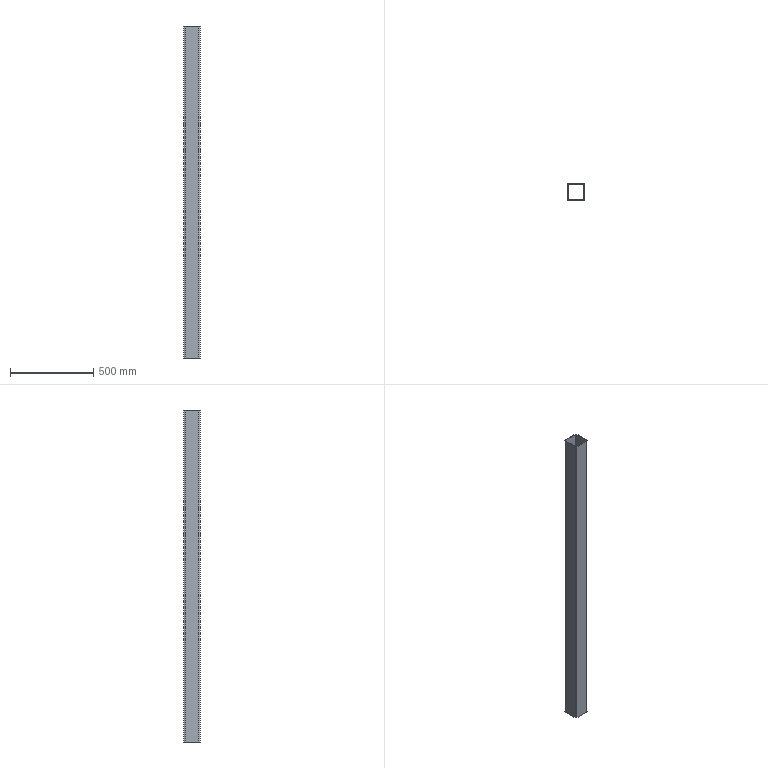Part | SolidWorks | features Extrusion 1, Shell 1 | 1 solid | 18 faces | box 100 x 100 x 2000 mm | volume 2986846 mm3 | plane 10 | cylinder 8 | commonest cylinder face diameters 8.4 x4 16.4 x4
STEP:
#1=CARTESIAN_POINT('',(-50.,-41.8,2000.));
#2=VERTEX_POINT('',#1);
#3=CARTESIAN_POINT('',(-41.8,-50.,2000.));
#4=VERTEX_POINT('',#3);
#5=CARTESIAN_POINT('',(-41.8,-41.8,2000.));
#6=DIRECTION('',(0.,0.,1.));
#7=DIRECTION('',(-1.,0.,0.));
#8=AXIS2_PLACEMENT_3D('',#5,#6,#7);
#9=CIRCLE('',#8,8.2);
#10=EDGE_CURVE('',#2,#4,#9,.T.);
#11=ORIENTED_EDGE('',*,*,#10,.T.);
#12=CARTESIAN_POINT('',(41.8,-50.,2000.));
#13=VERTEX_POINT('',#12);
#14=CARTESIAN_POINT('',(41.8,-50.,2000.));
#15=DIRECTION('',(1.,0.,0.));
#16=VECTOR('',#15,1000.);
#17=LINE('',#14,#16);
#18=EDGE_CURVE('',#4,#13,#17,.T.);
#19=ORIENTED_EDGE('',*,*,#18,.T.);
#20=CARTESIAN_POINT('',(50.,-41.8,2000.));
#21=VERTEX_POINT('',#20);
#22=CARTESIAN_POINT('',(41.8,-41.8,2000.));
#23=DIRECTION('',(0.,0.,1.));
#24=DIRECTION('',(-1.,0.,0.));
#25=AXIS2_PLACEMENT_3D('',#22,#23,#24);
#26=CIRCLE('',#25,8.2);
#27=EDGE_CURVE('',#13,#21,#26,.T.);
#28=ORIENTED_EDGE('',*,*,#27,.T.);
#29=CARTESIAN_POINT('',(50.,41.8,2000.));
#30=VERTEX_POINT('',#29);
#31=CARTESIAN_POINT('',(50.,41.8,2000.));
#32=DIRECTION('',(0.,1.,0.));
#33=VECTOR('',#32,1000.);
#34=LINE('',#31,#33);
#35=EDGE_CURVE('',#21,#30,#34,.T.);
#36=ORIENTED_EDGE('',*,*,#35,.T.);
#37=CARTESIAN_POINT('',(41.8,50.,2000.));
#38=VERTEX_POINT('',#37);
#39=CARTESIAN_POINT('',(41.8,41.8,2000.));
#40=DIRECTION('',(0.,0.,1.));
#41=DIRECTION('',(-1.,0.,0.));
#42=AXIS2_PLACEMENT_3D('',#39,#40,#41);
#43=CIRCLE('',#42,8.2);
#44=EDGE_CURVE('',#30,#38,#43,.T.);
#45=ORIENTED_EDGE('',*,*,#44,.T.);
#46=CARTESIAN_POINT('',(-41.8,50.,2000.));
#47=VERTEX_POINT('',#46);
#48=CARTESIAN_POINT('',(41.8,50.,2000.));
#49=DIRECTION('',(-1.,0.,0.));
#50=VECTOR('',#49,1000.);
#51=LINE('',#48,#50);
#52=EDGE_CURVE('',#38,#47,#51,.T.);
#53=ORIENTED_EDGE('',*,*,#52,.T.);
#54=CARTESIAN_POINT('',(-50.,41.8,2000.));
#55=VERTEX_POINT('',#54);
#56=CARTESIAN_POINT('',(-41.8,41.8,2000.));
#57=DIRECTION('',(0.,0.,1.));
#58=DIRECTION('',(-1.,0.,0.));
#59=AXIS2_PLACEMENT_3D('',#56,#57,#58);
#60=CIRCLE('',#59,8.2);
#61=EDGE_CURVE('',#47,#55,#60,.T.);
#62=ORIENTED_EDGE('',*,*,#61,.T.);
#63=CARTESIAN_POINT('',(-50.,41.8,2000.));
#64=DIRECTION('',(0.,-1.,0.));
#65=VECTOR('',#64,1000.);
#66=LINE('',#63,#65);
#67=EDGE_CURVE('',#55,#2,#66,.T.);
#68=ORIENTED_EDGE('',*,*,#67,.T.);
#69=EDGE_LOOP('',(#11,#19,#28,#36,#45,#53,#62,#68));
#70=FACE_OUTER_BOUND('',#69,.T.);
#71=CARTESIAN_POINT('',(-46.,-41.8,2000.));
#72=VERTEX_POINT('',#71);
#73=CARTESIAN_POINT('',(-41.8,-46.,2000.));
#74=VERTEX_POINT('',#73);
#75=CARTESIAN_POINT('',(-41.8,-41.8,2000.));
#76=DIRECTION('',(0.,0.,1.));
#77=DIRECTION('',(-1.,0.,0.));
#78=AXIS2_PLACEMENT_3D('',#75,#76,#77);
#79=CIRCLE('',#78,4.2);
#80=EDGE_CURVE('',#72,#74,#79,.T.);
#81=ORIENTED_EDGE('',*,*,#80,.F.);
#82=CARTESIAN_POINT('',(-46.,41.8,2000.));
#83=VERTEX_POINT('',#82);
#84=CARTESIAN_POINT('',(-46.,-41.8,2000.));
#85=DIRECTION('',(0.,-1.,0.));
#86=VECTOR('',#85,1000.);
#87=LINE('',#84,#86);
#88=EDGE_CURVE('',#83,#72,#87,.T.);
#89=ORIENTED_EDGE('',*,*,#88,.F.);
#90=CARTESIAN_POINT('',(-41.8,46.,2000.));
#91=VERTEX_POINT('',#90);
#92=CARTESIAN_POINT('',(-41.8,41.8,2000.));
#93=DIRECTION('',(0.,0.,1.));
#94=DIRECTION('',(-1.,0.,0.));
#95=AXIS2_PLACEMENT_3D('',#92,#93,#94);
#96=CIRCLE('',#95,4.2);
#97=EDGE_CURVE('',#91,#83,#96,.T.);
#98=ORIENTED_EDGE('',*,*,#97,.F.);
#99=CARTESIAN_POINT('',(41.8,46.,2000.));
#100=VERTEX_POINT('',#99);
#101=CARTESIAN_POINT('',(-41.8,46.,2000.));
#102=DIRECTION('',(-1.,0.,0.));
#103=VECTOR('',#102,1000.);
#104=LINE('',#101,#103);
#105=EDGE_CURVE('',#100,#91,#104,.T.);
#106=ORIENTED_EDGE('',*,*,#105,.F.);
#107=CARTESIAN_POINT('',(46.,41.8,2000.));
#108=VERTEX_POINT('',#107);
#109=CARTESIAN_POINT('',(41.8,41.8,2000.));
#110=DIRECTION('',(0.,0.,1.));
#111=DIRECTION('',(-1.,0.,0.));
#112=AXIS2_PLACEMENT_3D('',#109,#110,#111);
#113=CIRCLE('',#112,4.2);
#114=EDGE_CURVE('',#108,#100,#113,.T.);
#115=ORIENTED_EDGE('',*,*,#114,.F.);
#116=CARTESIAN_POINT('',(46.,-41.8,2000.));
#117=VERTEX_POINT('',#116);
#118=CARTESIAN_POINT('',(46.,-41.8,2000.));
#119=DIRECTION('',(0.,1.,0.));
#120=VECTOR('',#119,1000.);
#121=LINE('',#118,#120);
#122=EDGE_CURVE('',#117,#108,#121,.T.);
#123=ORIENTED_EDGE('',*,*,#122,.F.);
#124=CARTESIAN_POINT('',(41.8,-46.,2000.));
#125=VERTEX_POINT('',#124);
#126=CARTESIAN_POINT('',(41.8,-41.8,2000.));
#127=DIRECTION('',(0.,0.,1.));
#128=DIRECTION('',(-1.,0.,0.));
#129=AXIS2_PLACEMENT_3D('',#126,#127,#128);
#130=CIRCLE('',#129,4.2);
#131=EDGE_CURVE('',#125,#117,#130,.T.);
#132=ORIENTED_EDGE('',*,*,#131,.F.);
#133=CARTESIAN_POINT('',(-41.8,-46.,2000.));
#134=DIRECTION('',(1.,0.,0.));
#135=VECTOR('',#134,1000.);
#136=LINE('',#133,#135);
#137=EDGE_CURVE('',#74,#125,#136,.T.);
#138=ORIENTED_EDGE('',*,*,#137,.F.);
#139=EDGE_LOOP('',(#81,#89,#98,#106,#115,#123,#132,#138));
#140=FACE_BOUND('',#139,.T.);
#141=CARTESIAN_POINT('',(-41.8,-41.8,2000.));
#142=DIRECTION('',(0.,0.,-1.));
#143=DIRECTION('',(-1.,0.,0.));
#144=AXIS2_PLACEMENT_3D('',#141,#142,#143);
#145=PLANE('',#144);
#146=ADVANCED_FACE('',(#70,#140),#145,.F.);
#147=CARTESIAN_POINT('',(-50.,-41.8,0.));
#148=VERTEX_POINT('',#147);
#149=CARTESIAN_POINT('',(-41.8,-50.,0.));
#150=VERTEX_POINT('',#149);
#151=CARTESIAN_POINT('',(-41.8,-41.8,0.));
#152=DIRECTION('',(0.,0.,1.));
#153=DIRECTION('',(-1.,0.,0.));
#154=AXIS2_PLACEMENT_3D('',#151,#152,#153);
#155=CIRCLE('',#154,8.2);
#156=EDGE_CURVE('',#148,#150,#155,.T.);
#157=ORIENTED_EDGE('',*,*,#156,.F.);
#158=CARTESIAN_POINT('',(-50.,41.8,0.));
#159=VERTEX_POINT('',#158);
#160=CARTESIAN_POINT('',(-50.,41.8,0.));
#161=DIRECTION('',(0.,-1.,0.));
#162=VECTOR('',#161,1000.);
#163=LINE('',#160,#162);
#164=EDGE_CURVE('',#159,#148,#163,.T.);
#165=ORIENTED_EDGE('',*,*,#164,.F.);
#166=CARTESIAN_POINT('',(-41.8,50.,0.));
#167=VERTEX_POINT('',#166);
#168=CARTESIAN_POINT('',(-41.8,41.8,0.));
#169=DIRECTION('',(0.,0.,1.));
#170=DIRECTION('',(-1.,0.,0.));
#171=AXIS2_PLACEMENT_3D('',#168,#169,#170);
#172=CIRCLE('',#171,8.2);
#173=EDGE_CURVE('',#167,#159,#172,.T.);
#174=ORIENTED_EDGE('',*,*,#173,.F.);
#175=CARTESIAN_POINT('',(41.8,50.,0.));
#176=VERTEX_POINT('',#175);
#177=CARTESIAN_POINT('',(41.8,50.,0.));
#178=DIRECTION('',(-1.,0.,0.));
#179=VECTOR('',#178,1000.);
#180=LINE('',#177,#179);
#181=EDGE_CURVE('',#176,#167,#180,.T.);
#182=ORIENTED_EDGE('',*,*,#181,.F.);
#183=CARTESIAN_POINT('',(50.,41.8,0.));
#184=VERTEX_POINT('',#183);
#185=CARTESIAN_POINT('',(41.8,41.8,0.));
#186=DIRECTION('',(0.,0.,1.));
#187=DIRECTION('',(-1.,0.,0.));
#188=AXIS2_PLACEMENT_3D('',#185,#186,#187);
#189=CIRCLE('',#188,8.2);
#190=EDGE_CURVE('',#184,#176,#189,.T.);
#191=ORIENTED_EDGE('',*,*,#190,.F.);
#192=CARTESIAN_POINT('',(50.,-41.8,0.));
#193=VERTEX_POINT('',#192);
#194=CARTESIAN_POINT('',(50.,41.8,0.));
#195=DIRECTION('',(0.,1.,0.));
#196=VECTOR('',#195,1000.);
#197=LINE('',#194,#196);
#198=EDGE_CURVE('',#193,#184,#197,.T.);
#199=ORIENTED_EDGE('',*,*,#198,.F.);
#200=CARTESIAN_POINT('',(41.8,-50.,0.));
#201=VERTEX_POINT('',#200);
#202=CARTESIAN_POINT('',(41.8,-41.8,0.));
#203=DIRECTION('',(0.,0.,1.));
#204=DIRECTION('',(-1.,0.,0.));
#205=AXIS2_PLACEMENT_3D('',#202,#203,#204);
#206=CIRCLE('',#205,8.2);
#207=EDGE_CURVE('',#201,#193,#206,.T.);
#208=ORIENTED_EDGE('',*,*,#207,.F.);
#209=CARTESIAN_POINT('',(41.8,-50.,0.));
#210=DIRECTION('',(1.,0.,0.));
#211=VECTOR('',#210,1000.);
#212=LINE('',#209,#211);
#213=EDGE_CURVE('',#150,#201,#212,.T.);
#214=ORIENTED_EDGE('',*,*,#213,.F.);
#215=EDGE_LOOP('',(#157,#165,#174,#182,#191,#199,#208,#214));
#216=FACE_OUTER_BOUND('',#215,.T.);
#217=CARTESIAN_POINT('',(-46.,41.8,0.));
#218=VERTEX_POINT('',#217);
#219=CARTESIAN_POINT('',(-46.,-41.8,0.));
#220=VERTEX_POINT('',#219);
#221=CARTESIAN_POINT('',(-46.,-41.8,0.));
#222=DIRECTION('',(0.,-1.,0.));
#223=VECTOR('',#222,1000.);
#224=LINE('',#221,#223);
#225=EDGE_CURVE('',#218,#220,#224,.T.);
#226=ORIENTED_EDGE('',*,*,#225,.T.);
#227=CARTESIAN_POINT('',(-41.8,-46.,0.));
#228=VERTEX_POINT('',#227);
#229=CARTESIAN_POINT('',(-41.8,-41.8,0.));
#230=DIRECTION('',(0.,0.,1.));
#231=DIRECTION('',(-1.,0.,0.));
#232=AXIS2_PLACEMENT_3D('',#229,#230,#231);
#233=CIRCLE('',#232,4.2);
#234=EDGE_CURVE('',#220,#228,#233,.T.);
#235=ORIENTED_EDGE('',*,*,#234,.T.);
#236=CARTESIAN_POINT('',(41.8,-46.,0.));
#237=VERTEX_POINT('',#236);
#238=CARTESIAN_POINT('',(-41.8,-46.,0.));
#239=DIRECTION('',(1.,0.,0.));
#240=VECTOR('',#239,1000.);
#241=LINE('',#238,#240);
#242=EDGE_CURVE('',#228,#237,#241,.T.);
#243=ORIENTED_EDGE('',*,*,#242,.T.);
#244=CARTESIAN_POINT('',(46.,-41.8,0.));
#245=VERTEX_POINT('',#244);
#246=CARTESIAN_POINT('',(41.8,-41.8,0.));
#247=DIRECTION('',(0.,0.,1.));
#248=DIRECTION('',(-1.,0.,0.));
#249=AXIS2_PLACEMENT_3D('',#246,#247,#248);
#250=CIRCLE('',#249,4.2);
#251=EDGE_CURVE('',#237,#245,#250,.T.);
#252=ORIENTED_EDGE('',*,*,#251,.T.);
#253=CARTESIAN_POINT('',(46.,41.8,0.));
#254=VERTEX_POINT('',#253);
#255=CARTESIAN_POINT('',(46.,-41.8,0.));
#256=DIRECTION('',(0.,1.,0.));
#257=VECTOR('',#256,1000.);
#258=LINE('',#255,#257);
#259=EDGE_CURVE('',#245,#254,#258,.T.);
#260=ORIENTED_EDGE('',*,*,#259,.T.);
#261=CARTESIAN_POINT('',(41.8,46.,0.));
#262=VERTEX_POINT('',#261);
#263=CARTESIAN_POINT('',(41.8,41.8,0.));
#264=DIRECTION('',(0.,0.,1.));
#265=DIRECTION('',(-1.,0.,0.));
#266=AXIS2_PLACEMENT_3D('',#263,#264,#265);
#267=CIRCLE('',#266,4.2);
#268=EDGE_CURVE('',#254,#262,#267,.T.);
#269=ORIENTED_EDGE('',*,*,#268,.T.);
#270=CARTESIAN_POINT('',(-41.8,46.,0.));
#271=VERTEX_POINT('',#270);
#272=CARTESIAN_POINT('',(-41.8,46.,0.));
#273=DIRECTION('',(-1.,0.,0.));
#274=VECTOR('',#273,1000.);
#275=LINE('',#272,#274);
#276=EDGE_CURVE('',#262,#271,#275,.T.);
#277=ORIENTED_EDGE('',*,*,#276,.T.);
#278=CARTESIAN_POINT('',(-41.8,41.8,0.));
#279=DIRECTION('',(0.,0.,1.));
#280=DIRECTION('',(-1.,0.,0.));
#281=AXIS2_PLACEMENT_3D('',#278,#279,#280);
#282=CIRCLE('',#281,4.2);
#283=EDGE_CURVE('',#271,#218,#282,.T.);
#284=ORIENTED_EDGE('',*,*,#283,.T.);
#285=EDGE_LOOP('',(#226,#235,#243,#252,#260,#269,#277,#284));
#286=FACE_BOUND('',#285,.T.);
#287=CARTESIAN_POINT('',(-41.8,-41.8,0.));
#288=DIRECTION('',(0.,0.,-1.));
#289=DIRECTION('',(-1.,0.,0.));
#290=AXIS2_PLACEMENT_3D('',#287,#288,#289);
#291=PLANE('',#290);
#292=ADVANCED_FACE('',(#216,#286),#291,.T.);
#293=ORIENTED_EDGE('',*,*,#156,.T.);
#294=CARTESIAN_POINT('',(-41.8,-50.,2000.));
#295=DIRECTION('',(0.,0.,-1.));
#296=VECTOR('',#295,1000.);
#297=LINE('',#294,#296);
#298=EDGE_CURVE('',#4,#150,#297,.T.);
#299=ORIENTED_EDGE('',*,*,#298,.F.);
#300=ORIENTED_EDGE('',*,*,#10,.F.);
#301=CARTESIAN_POINT('',(-50.,-41.8,2000.));
#302=DIRECTION('',(0.,0.,-1.));
#303=VECTOR('',#302,1000.);
#304=LINE('',#301,#303);
#305=EDGE_CURVE('',#2,#148,#304,.T.);
#306=ORIENTED_EDGE('',*,*,#305,.T.);
#307=EDGE_LOOP('',(#293,#299,#300,#306));
#308=FACE_OUTER_BOUND('',#307,.T.);
#309=CARTESIAN_POINT('',(-41.8,-41.8,2000.));
#310=DIRECTION('',(0.,0.,-1.));
#311=DIRECTION('',(-1.,0.,0.));
#312=AXIS2_PLACEMENT_3D('',#309,#310,#311);
#313=CYLINDRICAL_SURFACE('',#312,8.2);
#314=ADVANCED_FACE('',(#308),#313,.T.);
#315=ORIENTED_EDGE('',*,*,#213,.T.);
#316=CARTESIAN_POINT('',(41.8,-50.,2000.));
#317=DIRECTION('',(0.,0.,-1.));
#318=VECTOR('',#317,1000.);
#319=LINE('',#316,#318);
#320=EDGE_CURVE('',#13,#201,#319,.T.);
#321=ORIENTED_EDGE('',*,*,#320,.F.);
#322=ORIENTED_EDGE('',*,*,#18,.F.);
#323=ORIENTED_EDGE('',*,*,#298,.T.);
#324=EDGE_LOOP('',(#315,#321,#322,#323));
#325=FACE_OUTER_BOUND('',#324,.T.);
#326=CARTESIAN_POINT('',(41.8,-50.,2000.));
#327=DIRECTION('',(0.,1.,0.));
#328=DIRECTION('',(-1.,0.,0.));
#329=AXIS2_PLACEMENT_3D('',#326,#327,#328);
#330=PLANE('',#329);
#331=ADVANCED_FACE('',(#325),#330,.F.);
#332=ORIENTED_EDGE('',*,*,#207,.T.);
#333=CARTESIAN_POINT('',(50.,-41.8,2000.));
#334=DIRECTION('',(0.,0.,-1.));
#335=VECTOR('',#334,1000.);
#336=LINE('',#333,#335);
#337=EDGE_CURVE('',#21,#193,#336,.T.);
#338=ORIENTED_EDGE('',*,*,#337,.F.);
#339=ORIENTED_EDGE('',*,*,#27,.F.);
#340=ORIENTED_EDGE('',*,*,#320,.T.);
#341=EDGE_LOOP('',(#332,#338,#339,#340));
#342=FACE_OUTER_BOUND('',#341,.T.);
#343=CARTESIAN_POINT('',(41.8,-41.8,2000.));
#344=DIRECTION('',(0.,0.,-1.));
#345=DIRECTION('',(-1.,0.,0.));
#346=AXIS2_PLACEMENT_3D('',#343,#344,#345);
#347=CYLINDRICAL_SURFACE('',#346,8.2);
#348=ADVANCED_FACE('',(#342),#347,.T.);
#349=ORIENTED_EDGE('',*,*,#198,.T.);
#350=CARTESIAN_POINT('',(50.,41.8,2000.));
#351=DIRECTION('',(0.,0.,-1.));
#352=VECTOR('',#351,1000.);
#353=LINE('',#350,#352);
#354=EDGE_CURVE('',#30,#184,#353,.T.);
#355=ORIENTED_EDGE('',*,*,#354,.F.);
#356=ORIENTED_EDGE('',*,*,#35,.F.);
#357=ORIENTED_EDGE('',*,*,#337,.T.);
#358=EDGE_LOOP('',(#349,#355,#356,#357));
#359=FACE_OUTER_BOUND('',#358,.T.);
#360=CARTESIAN_POINT('',(50.,41.8,2000.));
#361=DIRECTION('',(-1.,0.,0.));
#362=DIRECTION('',(0.,-1.,0.));
#363=AXIS2_PLACEMENT_3D('',#360,#361,#362);
#364=PLANE('',#363);
#365=ADVANCED_FACE('',(#359),#364,.F.);
#366=ORIENTED_EDGE('',*,*,#190,.T.);
#367=CARTESIAN_POINT('',(41.8,50.,2000.));
#368=DIRECTION('',(0.,0.,-1.));
#369=VECTOR('',#368,1000.);
#370=LINE('',#367,#369);
#371=EDGE_CURVE('',#38,#176,#370,.T.);
#372=ORIENTED_EDGE('',*,*,#371,.F.);
#373=ORIENTED_EDGE('',*,*,#44,.F.);
#374=ORIENTED_EDGE('',*,*,#354,.T.);
#375=EDGE_LOOP('',(#366,#372,#373,#374));
#376=FACE_OUTER_BOUND('',#375,.T.);
#377=CARTESIAN_POINT('',(41.8,41.8,2000.));
#378=DIRECTION('',(0.,0.,-1.));
#379=DIRECTION('',(-1.,0.,0.));
#380=AXIS2_PLACEMENT_3D('',#377,#378,#379);
#381=CYLINDRICAL_SURFACE('',#380,8.2);
#382=ADVANCED_FACE('',(#376),#381,.T.);
#383=ORIENTED_EDGE('',*,*,#181,.T.);
#384=CARTESIAN_POINT('',(-41.8,50.,2000.));
#385=DIRECTION('',(0.,0.,-1.));
#386=VECTOR('',#385,1000.);
#387=LINE('',#384,#386);
#388=EDGE_CURVE('',#47,#167,#387,.T.);
#389=ORIENTED_EDGE('',*,*,#388,.F.);
#390=ORIENTED_EDGE('',*,*,#52,.F.);
#391=ORIENTED_EDGE('',*,*,#371,.T.);
#392=EDGE_LOOP('',(#383,#389,#390,#391));
#393=FACE_OUTER_BOUND('',#392,.T.);
#394=CARTESIAN_POINT('',(41.8,50.,2000.));
#395=DIRECTION('',(0.,-1.,0.));
#396=DIRECTION('',(1.,0.,0.));
#397=AXIS2_PLACEMENT_3D('',#394,#395,#396);
#398=PLANE('',#397);
#399=ADVANCED_FACE('',(#393),#398,.F.);
#400=ORIENTED_EDGE('',*,*,#173,.T.);
#401=CARTESIAN_POINT('',(-50.,41.8,2000.));
#402=DIRECTION('',(0.,0.,-1.));
#403=VECTOR('',#402,1000.);
#404=LINE('',#401,#403);
#405=EDGE_CURVE('',#55,#159,#404,.T.);
#406=ORIENTED_EDGE('',*,*,#405,.F.);
#407=ORIENTED_EDGE('',*,*,#61,.F.);
#408=ORIENTED_EDGE('',*,*,#388,.T.);
#409=EDGE_LOOP('',(#400,#406,#407,#408));
#410=FACE_OUTER_BOUND('',#409,.T.);
#411=CARTESIAN_POINT('',(-41.8,41.8,2000.));
#412=DIRECTION('',(0.,0.,-1.));
#413=DIRECTION('',(-1.,0.,0.));
#414=AXIS2_PLACEMENT_3D('',#411,#412,#413);
#415=CYLINDRICAL_SURFACE('',#414,8.2);
#416=ADVANCED_FACE('',(#410),#415,.T.);
#417=ORIENTED_EDGE('',*,*,#164,.T.);
#418=ORIENTED_EDGE('',*,*,#305,.F.);
#419=ORIENTED_EDGE('',*,*,#67,.F.);
#420=ORIENTED_EDGE('',*,*,#405,.T.);
#421=EDGE_LOOP('',(#417,#418,#419,#420));
#422=FACE_OUTER_BOUND('',#421,.T.);
#423=CARTESIAN_POINT('',(-50.,41.8,2000.));
#424=DIRECTION('',(1.,0.,0.));
#425=DIRECTION('',(0.,1.,0.));
#426=AXIS2_PLACEMENT_3D('',#423,#424,#425);
#427=PLANE('',#426);
#428=ADVANCED_FACE('',(#422),#427,.F.);
#429=ORIENTED_EDGE('',*,*,#234,.F.);
#430=CARTESIAN_POINT('',(-46.,-41.8,2000.));
#431=DIRECTION('',(0.,0.,-1.));
#432=VECTOR('',#431,1000.);
#433=LINE('',#430,#432);
#434=EDGE_CURVE('',#72,#220,#433,.T.);
#435=ORIENTED_EDGE('',*,*,#434,.F.);
#436=ORIENTED_EDGE('',*,*,#80,.T.);
#437=CARTESIAN_POINT('',(-41.8,-46.,2000.));
#438=DIRECTION('',(0.,0.,-1.));
#439=VECTOR('',#438,1000.);
#440=LINE('',#437,#439);
#441=EDGE_CURVE('',#74,#228,#440,.T.);
#442=ORIENTED_EDGE('',*,*,#441,.T.);
#443=EDGE_LOOP('',(#429,#435,#436,#442));
#444=FACE_OUTER_BOUND('',#443,.T.);
#445=CARTESIAN_POINT('',(-41.8,-41.8,2000.));
#446=DIRECTION('',(0.,0.,-1.));
#447=DIRECTION('',(-1.,0.,0.));
#448=AXIS2_PLACEMENT_3D('',#445,#446,#447);
#449=CYLINDRICAL_SURFACE('',#448,4.2);
#450=ADVANCED_FACE('',(#444),#449,.F.);
#451=ORIENTED_EDGE('',*,*,#242,.F.);
#452=ORIENTED_EDGE('',*,*,#441,.F.);
#453=ORIENTED_EDGE('',*,*,#137,.T.);
#454=CARTESIAN_POINT('',(41.8,-46.,2000.));
#455=DIRECTION('',(0.,0.,-1.));
#456=VECTOR('',#455,1000.);
#457=LINE('',#454,#456);
#458=EDGE_CURVE('',#125,#237,#457,.T.);
#459=ORIENTED_EDGE('',*,*,#458,.T.);
#460=EDGE_LOOP('',(#451,#452,#453,#459));
#461=FACE_OUTER_BOUND('',#460,.T.);
#462=CARTESIAN_POINT('',(41.8,-46.,2000.));
#463=DIRECTION('',(0.,1.,0.));
#464=DIRECTION('',(-1.,0.,0.));
#465=AXIS2_PLACEMENT_3D('',#462,#463,#464);
#466=PLANE('',#465);
#467=ADVANCED_FACE('',(#461),#466,.T.);
#468=ORIENTED_EDGE('',*,*,#251,.F.);
#469=ORIENTED_EDGE('',*,*,#458,.F.);
#470=ORIENTED_EDGE('',*,*,#131,.T.);
#471=CARTESIAN_POINT('',(46.,-41.8,2000.));
#472=DIRECTION('',(0.,0.,-1.));
#473=VECTOR('',#472,1000.);
#474=LINE('',#471,#473);
#475=EDGE_CURVE('',#117,#245,#474,.T.);
#476=ORIENTED_EDGE('',*,*,#475,.T.);
#477=EDGE_LOOP('',(#468,#469,#470,#476));
#478=FACE_OUTER_BOUND('',#477,.T.);
#479=CARTESIAN_POINT('',(41.8,-41.8,2000.));
#480=DIRECTION('',(0.,0.,-1.));
#481=DIRECTION('',(-1.,0.,0.));
#482=AXIS2_PLACEMENT_3D('',#479,#480,#481);
#483=CYLINDRICAL_SURFACE('',#482,4.2);
#484=ADVANCED_FACE('',(#478),#483,.F.);
#485=ORIENTED_EDGE('',*,*,#259,.F.);
#486=ORIENTED_EDGE('',*,*,#475,.F.);
#487=ORIENTED_EDGE('',*,*,#122,.T.);
#488=CARTESIAN_POINT('',(46.,41.8,2000.));
#489=DIRECTION('',(0.,0.,-1.));
#490=VECTOR('',#489,1000.);
#491=LINE('',#488,#490);
#492=EDGE_CURVE('',#108,#254,#491,.T.);
#493=ORIENTED_EDGE('',*,*,#492,.T.);
#494=EDGE_LOOP('',(#485,#486,#487,#493));
#495=FACE_OUTER_BOUND('',#494,.T.);
#496=CARTESIAN_POINT('',(46.,41.8,2000.));
#497=DIRECTION('',(-1.,0.,0.));
#498=DIRECTION('',(0.,-1.,0.));
#499=AXIS2_PLACEMENT_3D('',#496,#497,#498);
#500=PLANE('',#499);
#501=ADVANCED_FACE('',(#495),#500,.T.);
#502=ORIENTED_EDGE('',*,*,#268,.F.);
#503=ORIENTED_EDGE('',*,*,#492,.F.);
#504=ORIENTED_EDGE('',*,*,#114,.T.);
#505=CARTESIAN_POINT('',(41.8,46.,2000.));
#506=DIRECTION('',(0.,0.,-1.));
#507=VECTOR('',#506,1000.);
#508=LINE('',#505,#507);
#509=EDGE_CURVE('',#100,#262,#508,.T.);
#510=ORIENTED_EDGE('',*,*,#509,.T.);
#511=EDGE_LOOP('',(#502,#503,#504,#510));
#512=FACE_OUTER_BOUND('',#511,.T.);
#513=CARTESIAN_POINT('',(41.8,41.8,2000.));
#514=DIRECTION('',(0.,0.,-1.));
#515=DIRECTION('',(-1.,0.,0.));
#516=AXIS2_PLACEMENT_3D('',#513,#514,#515);
#517=CYLINDRICAL_SURFACE('',#516,4.2);
#518=ADVANCED_FACE('',(#512),#517,.F.);
#519=ORIENTED_EDGE('',*,*,#276,.F.);
#520=ORIENTED_EDGE('',*,*,#509,.F.);
#521=ORIENTED_EDGE('',*,*,#105,.T.);
#522=CARTESIAN_POINT('',(-41.8,46.,2000.));
#523=DIRECTION('',(0.,0.,-1.));
#524=VECTOR('',#523,1000.);
#525=LINE('',#522,#524);
#526=EDGE_CURVE('',#91,#271,#525,.T.);
#527=ORIENTED_EDGE('',*,*,#526,.T.);
#528=EDGE_LOOP('',(#519,#520,#521,#527));
#529=FACE_OUTER_BOUND('',#528,.T.);
#530=CARTESIAN_POINT('',(41.8,46.,2000.));
#531=DIRECTION('',(0.,-1.,0.));
#532=DIRECTION('',(1.,0.,0.));
#533=AXIS2_PLACEMENT_3D('',#530,#531,#532);
#534=PLANE('',#533);
#535=ADVANCED_FACE('',(#529),#534,.T.);
#536=ORIENTED_EDGE('',*,*,#283,.F.);
#537=ORIENTED_EDGE('',*,*,#526,.F.);
#538=ORIENTED_EDGE('',*,*,#97,.T.);
#539=CARTESIAN_POINT('',(-46.,41.8,2000.));
#540=DIRECTION('',(0.,0.,-1.));
#541=VECTOR('',#540,1000.);
#542=LINE('',#539,#541);
#543=EDGE_CURVE('',#83,#218,#542,.T.);
#544=ORIENTED_EDGE('',*,*,#543,.T.);
#545=EDGE_LOOP('',(#536,#537,#538,#544));
#546=FACE_OUTER_BOUND('',#545,.T.);
#547=CARTESIAN_POINT('',(-41.8,41.8,2000.));
#548=DIRECTION('',(0.,0.,-1.));
#549=DIRECTION('',(-1.,0.,0.));
#550=AXIS2_PLACEMENT_3D('',#547,#548,#549);
#551=CYLINDRICAL_SURFACE('',#550,4.2);
#552=ADVANCED_FACE('',(#546),#551,.F.);
#553=ORIENTED_EDGE('',*,*,#225,.F.);
#554=ORIENTED_EDGE('',*,*,#543,.F.);
#555=ORIENTED_EDGE('',*,*,#88,.T.);
#556=ORIENTED_EDGE('',*,*,#434,.T.);
#557=EDGE_LOOP('',(#553,#554,#555,#556));
#558=FACE_OUTER_BOUND('',#557,.T.);
#559=CARTESIAN_POINT('',(-46.,41.8,2000.));
#560=DIRECTION('',(1.,0.,0.));
#561=DIRECTION('',(0.,1.,0.));
#562=AXIS2_PLACEMENT_3D('',#559,#560,#561);
#563=PLANE('',#562);
#564=ADVANCED_FACE('',(#558),#563,.T.);
#565=CLOSED_SHELL('',(#146,#292,#314,#331,#348,#365,#382,#399,#416,#428,#450,#467,#484,#501,#518,#535,#552,#564));
#566=MANIFOLD_SOLID_BREP('',#565);
#567=CARTESIAN_POINT('',(0.,0.,0.));
#568=DIRECTION('',(0.,0.,1.));
#569=DIRECTION('',(1.,0.,0.));
#570=AXIS2_PLACEMENT_3D('',#567,#568,#569);
#571=(LENGTH_UNIT()NAMED_UNIT(*)SI_UNIT(.MILLI.,.METRE.));
#572=UNCERTAINTY_MEASURE_WITH_UNIT(LENGTH_MEASURE(0.00001),#571,'','');
#573=(NAMED_UNIT(*)PLANE_ANGLE_UNIT()SI_UNIT($,.RADIAN.));
#574=(NAMED_UNIT(*)SI_UNIT($,.STERADIAN.)SOLID_ANGLE_UNIT());
#575=(GEOMETRIC_REPRESENTATION_CONTEXT(3)GLOBAL_UNCERTAINTY_ASSIGNED_CONTEXT((#572))GLOBAL_UNIT_ASSIGNED_CONTEXT((#571,#573,#574))REPRESENTATION_CONTEXT('',''));
#576=ADVANCED_BREP_SHAPE_REPRESENTATION('',(#566,#570),#575);